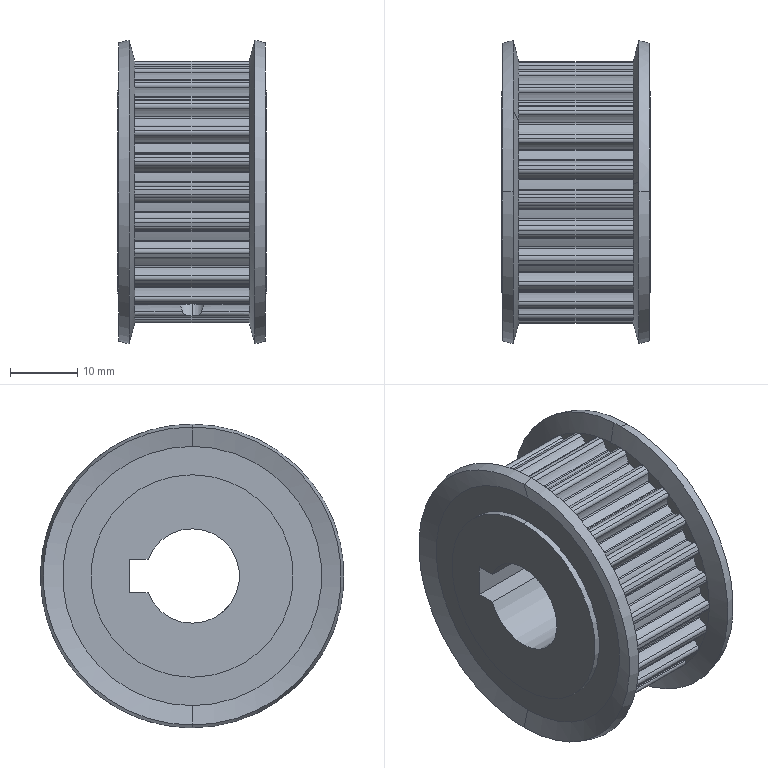Part | STEP file | C-HTPA25S5M150-A-N14^Pull-feed drive assembly | 1 solid | 288 faces | box 22 x 45 x 45 mm | volume 20511 mm3 | cylinder 219 | plane 57 | cone 12 | commonest cylinder face diameters 0.5 x54 6.55 x54 1.1 x50 35.29 x27 38.83 x25 4.134 x4